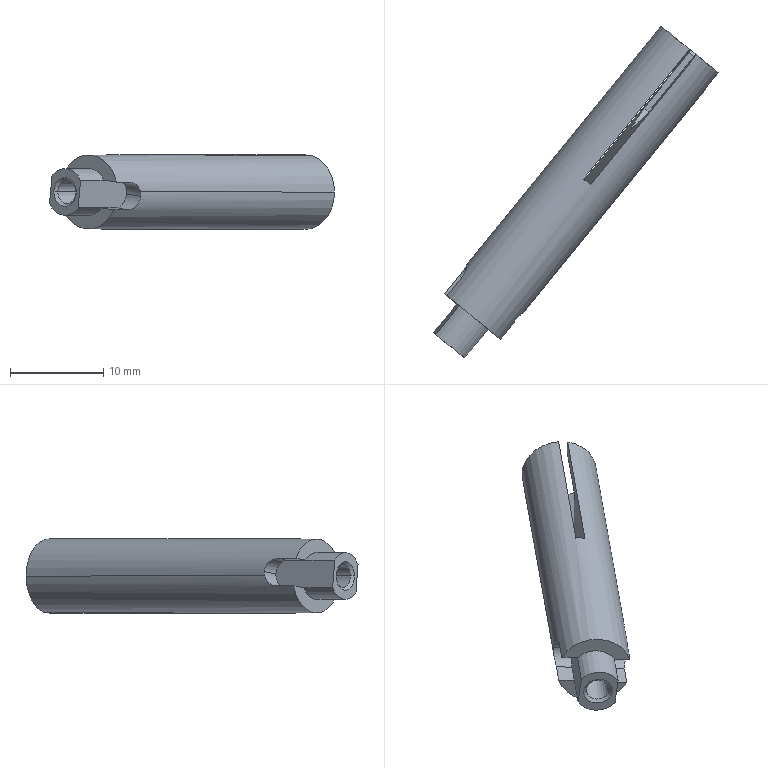Part | SolidWorks | features BaseBody 1 | 1 solid | 39 faces | box 30.645 x 35.694 x 8 mm | volume 1475 mm3 | plane 14 | cylinder 13 | cone 10 | spline 2 | commonest cylinder face diameters 3 x4 6 x3 2.5 x2 5 x2 8 x2
STEP:
#1=CARTESIAN_POINT('',(540.128,-144.913,299.195));
#2=VERTEX_POINT('',#1);
#3=CARTESIAN_POINT('',(538.707,-143.757,300.301));
#4=VERTEX_POINT('',#3);
#5=CARTESIAN_POINT('',(539.158,-144.124,299.195));
#6=DIRECTION('',(-0.6309,-0.7758,0.000000012));
#7=DIRECTION('',(0.7758,-0.6309,0.));
#8=AXIS2_PLACEMENT_3D('',#5,#6,#7);
#9=CIRCLE('',#8,1.25);
#10=EDGE_CURVE('',#2,#4,#9,.T.);
#11=ORIENTED_EDGE('',*,*,#10,.T.);
#12=CARTESIAN_POINT('',(539.969,-142.205,300.301));
#13=VERTEX_POINT('',#12);
#14=CARTESIAN_POINT('',(538.707,-143.757,300.301));
#15=CARTESIAN_POINT('',(539.969,-142.205,300.301));
#16=B_SPLINE_CURVE_WITH_KNOTS('',1,(#14,#15),.UNSPECIFIED.,.F.,.F.,(2,2),(0.,1.),.UNSPECIFIED.);
#17=EDGE_CURVE('',#4,#13,#16,.T.);
#18=ORIENTED_EDGE('',*,*,#17,.T.);
#19=CARTESIAN_POINT('',(541.39,-143.361,299.195));
#20=VERTEX_POINT('',#19);
#21=CARTESIAN_POINT('',(540.42,-142.572,299.195));
#22=DIRECTION('',(-0.6309,-0.7758,0.000000012));
#23=DIRECTION('',(0.7758,-0.6309,0.));
#24=AXIS2_PLACEMENT_3D('',#21,#22,#23);
#25=CIRCLE('',#24,1.25);
#26=EDGE_CURVE('',#20,#13,#25,.T.);
#27=ORIENTED_EDGE('',*,*,#26,.F.);
#28=CARTESIAN_POINT('',(540.871,-142.939,298.088));
#29=VERTEX_POINT('',#28);
#30=CARTESIAN_POINT('',(540.42,-142.572,299.195));
#31=DIRECTION('',(-0.6309,-0.7758,0.000000012));
#32=DIRECTION('',(0.7758,-0.6309,0.));
#33=AXIS2_PLACEMENT_3D('',#30,#31,#32);
#34=CIRCLE('',#33,1.25);
#35=EDGE_CURVE('',#29,#20,#34,.T.);
#36=ORIENTED_EDGE('',*,*,#35,.F.);
#37=CARTESIAN_POINT('',(539.609,-144.491,298.088));
#38=VERTEX_POINT('',#37);
#39=CARTESIAN_POINT('',(539.609,-144.491,298.088));
#40=CARTESIAN_POINT('',(540.871,-142.939,298.088));
#41=B_SPLINE_CURVE_WITH_KNOTS('',1,(#39,#40),.UNSPECIFIED.,.F.,.F.,(2,2),(0.,1.),.UNSPECIFIED.);
#42=EDGE_CURVE('',#38,#29,#41,.T.);
#43=ORIENTED_EDGE('',*,*,#42,.F.);
#44=CARTESIAN_POINT('',(539.158,-144.124,299.195));
#45=DIRECTION('',(-0.6309,-0.7758,0.000000012));
#46=DIRECTION('',(0.7758,-0.6309,0.));
#47=AXIS2_PLACEMENT_3D('',#44,#45,#46);
#48=CIRCLE('',#47,1.25);
#49=EDGE_CURVE('',#38,#2,#48,.T.);
#50=ORIENTED_EDGE('',*,*,#49,.T.);
#51=EDGE_LOOP('',(#11,#18,#27,#36,#43,#50));
#52=FACE_OUTER_BOUND('',#51,.T.);
#53=CARTESIAN_POINT('',(539.609,-144.491,298.088));
#54=CARTESIAN_POINT('',(541.326,-145.887,299.252));
#55=CARTESIAN_POINT('',(540.423,-145.153,301.464));
#56=CARTESIAN_POINT('',(538.707,-143.757,300.301));
#57=CARTESIAN_POINT('',(536.99,-142.361,299.138));
#58=CARTESIAN_POINT('',(537.892,-143.095,296.925));
#59=CARTESIAN_POINT('',(539.609,-144.491,298.088));
#60=CARTESIAN_POINT('',(540.871,-142.939,298.088));
#61=CARTESIAN_POINT('',(542.588,-144.335,299.252));
#62=CARTESIAN_POINT('',(541.685,-143.601,301.464));
#63=CARTESIAN_POINT('',(539.969,-142.205,300.301));
#64=CARTESIAN_POINT('',(538.252,-140.809,299.138));
#65=CARTESIAN_POINT('',(539.154,-141.543,296.925));
#66=CARTESIAN_POINT('',(540.871,-142.939,298.088));
#67=(BOUNDED_SURFACE()B_SPLINE_SURFACE(1,3,((#53,#54,#55,#56,#57,#58,#59),(#60,#61,#62,#63,#64,#65,#66)),.UNSPECIFIED.,.F.,.T.,.F.)B_SPLINE_SURFACE_WITH_KNOTS((2,2),(4,3,4),(0.,1.),(0.,0.5,1.),.UNSPECIFIED.)GEOMETRIC_REPRESENTATION_ITEM()RATIONAL_B_SPLINE_SURFACE(((1.,0.3333,0.3333,1.,0.3333,0.3333,1.),(1.,0.3333,0.3333,1.,0.3333,0.3333,1.)))REPRESENTATION_ITEM('')SURFACE());
#68=ADVANCED_FACE('',(#52),#67,.F.);
#69=CARTESIAN_POINT('',(538.678,-150.822,300.267));
#70=VERTEX_POINT('',#69);
#71=CARTESIAN_POINT('',(539.694,-149.805,299.195));
#72=VERTEX_POINT('',#71);
#73=CARTESIAN_POINT('',(538.678,-150.822,300.267));
#74=CARTESIAN_POINT('',(538.779,-150.697,300.267));
#75=CARTESIAN_POINT('',(538.884,-150.58,300.241));
#76=CARTESIAN_POINT('',(539.097,-150.361,300.137));
#77=CARTESIAN_POINT('',(539.2,-150.264,300.061));
#78=CARTESIAN_POINT('',(539.39,-150.09,299.868));
#79=CARTESIAN_POINT('',(539.474,-150.017,299.753));
#80=CARTESIAN_POINT('',(539.612,-149.891,299.491));
#81=CARTESIAN_POINT('',(539.664,-149.842,299.347));
#82=CARTESIAN_POINT('',(539.694,-149.805,299.195));
#83=B_SPLINE_CURVE_WITH_KNOTS('',3,(#73,#74,#75,#76,#77,#78,#79,#80,#81,#82),.UNSPECIFIED.,.F.,.F.,(4,2,2,2,4),(0.,0.0004777,0.0009554,0.001433,0.001911),.UNSPECIFIED.);
#84=EDGE_CURVE('',#70,#72,#83,.T.);
#85=ORIENTED_EDGE('',*,*,#84,.T.);
#86=CARTESIAN_POINT('',(560.558,-124.148,299.195));
#87=VERTEX_POINT('',#86);
#88=CARTESIAN_POINT('',(537.214,-152.854,299.195));
#89=DIRECTION('',(0.6309,0.7758,-0.000000012));
#90=VECTOR('',#89,1000.);
#91=LINE('',#88,#90);
#92=EDGE_CURVE('',#72,#87,#91,.T.);
#93=ORIENTED_EDGE('',*,*,#92,.T.);
#94=CARTESIAN_POINT('',(558.187,-122.22,303.082));
#95=VERTEX_POINT('',#94);
#96=CARTESIAN_POINT('',(557.455,-121.625,299.195));
#97=DIRECTION('',(-0.6309,-0.7758,0.000000012));
#98=DIRECTION('',(-0.7758,0.6309,0.));
#99=AXIS2_PLACEMENT_3D('',#96,#97,#98);
#100=CIRCLE('',#99,4.);
#101=EDGE_CURVE('',#87,#95,#100,.T.);
#102=ORIENTED_EDGE('',*,*,#101,.T.);
#103=CARTESIAN_POINT('',(546.831,-136.185,303.082));
#104=VERTEX_POINT('',#103);
#105=CARTESIAN_POINT('',(534.843,-150.926,303.082));
#106=DIRECTION('',(-0.6309,-0.7758,0.000000012));
#107=VECTOR('',#106,1000.);
#108=LINE('',#105,#107);
#109=EDGE_CURVE('',#95,#104,#108,.T.);
#110=ORIENTED_EDGE('',*,*,#109,.T.);
#111=CARTESIAN_POINT('',(546.06,-135.558,303.194));
#112=VERTEX_POINT('',#111);
#113=CARTESIAN_POINT('',(546.098,-135.59,299.195));
#114=DIRECTION('',(-0.6309,-0.7758,0.000000012));
#115=DIRECTION('',(-0.7758,0.6309,0.));
#116=AXIS2_PLACEMENT_3D('',#113,#114,#115);
#117=CIRCLE('',#116,4.);
#118=EDGE_CURVE('',#104,#112,#117,.T.);
#119=ORIENTED_EDGE('',*,*,#118,.T.);
#120=CARTESIAN_POINT('',(557.416,-121.593,303.194));
#121=VERTEX_POINT('',#120);
#122=CARTESIAN_POINT('',(534.072,-150.299,303.194));
#123=DIRECTION('',(0.6309,0.7758,-0.000000012));
#124=VECTOR('',#123,1000.);
#125=LINE('',#122,#124);
#126=EDGE_CURVE('',#112,#121,#125,.T.);
#127=ORIENTED_EDGE('',*,*,#126,.T.);
#128=CARTESIAN_POINT('',(554.352,-119.101,299.195));
#129=VERTEX_POINT('',#128);
#130=CARTESIAN_POINT('',(557.455,-121.625,299.195));
#131=DIRECTION('',(-0.6309,-0.7758,0.000000012));
#132=DIRECTION('',(-0.7758,0.6309,0.));
#133=AXIS2_PLACEMENT_3D('',#130,#131,#132);
#134=CIRCLE('',#133,4.);
#135=EDGE_CURVE('',#121,#129,#134,.T.);
#136=ORIENTED_EDGE('',*,*,#135,.T.);
#137=CARTESIAN_POINT('',(533.487,-144.757,299.195));
#138=VERTEX_POINT('',#137);
#139=CARTESIAN_POINT('',(531.007,-147.807,299.195));
#140=DIRECTION('',(0.6309,0.7758,-0.000000012));
#141=VECTOR('',#140,1000.);
#142=LINE('',#139,#141);
#143=EDGE_CURVE('',#138,#129,#142,.T.);
#144=ORIENTED_EDGE('',*,*,#143,.F.);
#145=CARTESIAN_POINT('',(533.551,-144.72,299.645));
#146=VERTEX_POINT('',#145);
#147=CARTESIAN_POINT('',(533.487,-144.757,299.195));
#148=CARTESIAN_POINT('',(533.516,-144.722,299.339));
#149=CARTESIAN_POINT('',(533.537,-144.709,299.492));
#150=CARTESIAN_POINT('',(533.551,-144.72,299.645));
#151=B_SPLINE_CURVE_WITH_KNOTS('',3,(#147,#148,#149,#150),.UNSPECIFIED.,.F.,.F.,(4,4),(0.0007269,0.001182),.UNSPECIFIED.);
#152=EDGE_CURVE('',#138,#146,#151,.T.);
#153=ORIENTED_EDGE('',*,*,#152,.T.);
#154=CARTESIAN_POINT('',(532.96,-146.173,301.103));
#155=VERTEX_POINT('',#154);
#156=CARTESIAN_POINT('',(533.551,-144.72,299.645));
#157=CARTESIAN_POINT('',(533.559,-144.727,299.745));
#158=CARTESIAN_POINT('',(533.565,-144.744,299.842));
#159=CARTESIAN_POINT('',(533.568,-144.796,300.032));
#160=CARTESIAN_POINT('',(533.566,-144.833,300.126));
#161=CARTESIAN_POINT('',(533.549,-144.965,300.391));
#162=CARTESIAN_POINT('',(533.522,-145.086,300.551));
#163=CARTESIAN_POINT('',(533.431,-145.365,300.815));
#164=CARTESIAN_POINT('',(533.366,-145.526,300.921));
#165=CARTESIAN_POINT('',(533.195,-145.85,301.064));
#166=CARTESIAN_POINT('',(533.087,-146.018,301.103));
#167=CARTESIAN_POINT('',(532.96,-146.173,301.103));
#168=B_SPLINE_CURVE_WITH_KNOTS('',3,(#156,#157,#158,#159,#160,#161,#162,#163,#164,#165,#166,#167),.UNSPECIFIED.,.F.,.F.,(4,2,2,2,2,4),(0.001182,0.001478,0.001774,0.002365,0.002957,0.003548),.UNSPECIFIED.);
#169=EDGE_CURVE('',#146,#155,#168,.T.);
#170=ORIENTED_EDGE('',*,*,#169,.T.);
#171=CARTESIAN_POINT('',(531.383,-148.113,301.103));
#172=VERTEX_POINT('',#171);
#173=CARTESIAN_POINT('',(531.383,-148.113,301.103));
#174=DIRECTION('',(-0.6309,-0.7758,0.000000012));
#175=VECTOR('',#174,1000.);
#176=LINE('',#173,#175);
#177=EDGE_CURVE('',#155,#172,#176,.T.);
#178=ORIENTED_EDGE('',*,*,#177,.T.);
#179=CARTESIAN_POINT('',(537.1,-152.762,300.267));
#180=VERTEX_POINT('',#179);
#181=CARTESIAN_POINT('',(534.111,-150.331,299.195));
#182=DIRECTION('',(0.6309,0.7758,-0.000000012));
#183=DIRECTION('',(-0.7758,0.6309,0.));
#184=AXIS2_PLACEMENT_3D('',#181,#182,#183);
#185=CIRCLE('',#184,4.);
#186=EDGE_CURVE('',#172,#180,#185,.T.);
#187=ORIENTED_EDGE('',*,*,#186,.T.);
#188=CARTESIAN_POINT('',(537.1,-152.762,300.267));
#189=DIRECTION('',(0.6309,0.7758,-0.000000012));
#190=VECTOR('',#189,1000.);
#191=LINE('',#188,#190);
#192=EDGE_CURVE('',#180,#70,#191,.T.);
#193=ORIENTED_EDGE('',*,*,#192,.T.);
#194=EDGE_LOOP('',(#85,#93,#102,#110,#119,#127,#136,#144,#153,#170,#178,#187,#193));
#195=FACE_OUTER_BOUND('',#194,.T.);
#196=CARTESIAN_POINT('',(534.111,-150.331,299.195));
#197=DIRECTION('',(0.6309,0.7758,-0.000000012));
#198=DIRECTION('',(-0.7758,0.6309,0.));
#199=AXIS2_PLACEMENT_3D('',#196,#197,#198);
#200=CYLINDRICAL_SURFACE('',#199,4.);
#201=ADVANCED_FACE('',(#195),#200,.T.);
#202=ORIENTED_EDGE('',*,*,#169,.F.);
#203=CARTESIAN_POINT('',(535.092,-145.974,299.42));
#204=VERTEX_POINT('',#203);
#205=CARTESIAN_POINT('',(534.08,-145.151,299.568));
#206=DIRECTION('',(0.7709,-0.6269,-0.1126));
#207=VECTOR('',#206,1000.);
#208=LINE('',#205,#207);
#209=EDGE_CURVE('',#146,#204,#208,.T.);
#210=ORIENTED_EDGE('',*,*,#209,.T.);
#211=CARTESIAN_POINT('',(534.277,-147.244,300.91));
#212=VERTEX_POINT('',#211);
#213=CARTESIAN_POINT('',(534.146,-147.137,299.42));
#214=DIRECTION('',(-0.7709,0.6269,0.1126));
#215=DIRECTION('',(0.6309,0.7758,0.));
#216=AXIS2_PLACEMENT_3D('',#213,#214,#215);
#217=CIRCLE('',#216,1.5);
#218=EDGE_CURVE('',#212,#204,#217,.T.);
#219=ORIENTED_EDGE('',*,*,#218,.F.);
#220=CARTESIAN_POINT('',(534.277,-147.244,300.91));
#221=DIRECTION('',(-0.7709,0.6269,0.1126));
#222=VECTOR('',#221,1000.);
#223=LINE('',#220,#222);
#224=EDGE_CURVE('',#212,#155,#223,.T.);
#225=ORIENTED_EDGE('',*,*,#224,.T.);
#226=EDGE_LOOP('',(#202,#210,#219,#225));
#227=FACE_OUTER_BOUND('',#226,.T.);
#228=CARTESIAN_POINT('',(533.134,-146.314,299.568));
#229=DIRECTION('',(0.7709,-0.6269,-0.1126));
#230=DIRECTION('',(0.6309,0.7758,0.));
#231=AXIS2_PLACEMENT_3D('',#228,#229,#230);
#232=CYLINDRICAL_SURFACE('',#231,1.5);
#233=ADVANCED_FACE('',(#227),#232,.F.);
#234=CARTESIAN_POINT('',(538.176,-148.481,298.969));
#235=VERTEX_POINT('',#234);
#236=CARTESIAN_POINT('',(537.361,-149.752,300.46));
#237=VERTEX_POINT('',#236);
#238=CARTESIAN_POINT('',(537.23,-149.645,298.969));
#239=DIRECTION('',(0.7709,-0.6269,-0.1126));
#240=DIRECTION('',(0.6309,0.7758,0.));
#241=AXIS2_PLACEMENT_3D('',#238,#239,#240);
#242=CIRCLE('',#241,1.5);
#243=EDGE_CURVE('',#235,#237,#242,.T.);
#244=ORIENTED_EDGE('',*,*,#243,.F.);
#245=CARTESIAN_POINT('',(539.718,-149.735,298.744));
#246=VERTEX_POINT('',#245);
#247=CARTESIAN_POINT('',(538.53,-148.769,298.918));
#248=DIRECTION('',(0.7709,-0.6269,-0.1126));
#249=VECTOR('',#248,1000.);
#250=LINE('',#247,#249);
#251=EDGE_CURVE('',#235,#246,#250,.T.);
#252=ORIENTED_EDGE('',*,*,#251,.T.);
#253=CARTESIAN_POINT('',(539.694,-149.805,299.195));
#254=CARTESIAN_POINT('',(539.723,-149.77,299.049));
#255=CARTESIAN_POINT('',(539.731,-149.746,298.897));
#256=CARTESIAN_POINT('',(539.718,-149.735,298.744));
#257=B_SPLINE_CURVE_WITH_KNOTS('',3,(#253,#254,#255,#256),.UNSPECIFIED.,.F.,.F.,(4,4),(0.001911,0.002365),.UNSPECIFIED.);
#258=EDGE_CURVE('',#72,#246,#257,.T.);
#259=ORIENTED_EDGE('',*,*,#258,.F.);
#260=ORIENTED_EDGE('',*,*,#84,.F.);
#261=CARTESIAN_POINT('',(537.714,-150.039,300.408));
#262=DIRECTION('',(0.7709,-0.6269,-0.1126));
#263=VECTOR('',#262,1000.);
#264=LINE('',#261,#263);
#265=EDGE_CURVE('',#237,#70,#264,.T.);
#266=ORIENTED_EDGE('',*,*,#265,.F.);
#267=EDGE_LOOP('',(#244,#252,#259,#260,#266));
#268=FACE_OUTER_BOUND('',#267,.T.);
#269=CARTESIAN_POINT('',(537.583,-149.933,298.918));
#270=DIRECTION('',(0.7709,-0.6269,-0.1126));
#271=DIRECTION('',(0.6309,0.7758,0.));
#272=AXIS2_PLACEMENT_3D('',#269,#270,#271);
#273=CYLINDRICAL_SURFACE('',#272,1.5);
#274=ADVANCED_FACE('',(#268),#273,.F.);
#275=CARTESIAN_POINT('',(557.91,-122.381,302.077));
#276=VERTEX_POINT('',#275);
#277=CARTESIAN_POINT('',(559.593,-123.75,299.195));
#278=VERTEX_POINT('',#277);
#279=CARTESIAN_POINT('',(557.266,-121.857,299.195));
#280=DIRECTION('',(0.6309,0.7758,-0.000000012));
#281=DIRECTION('',(0.361,-0.2936,-0.8851));
#282=AXIS2_PLACEMENT_3D('',#279,#280,#281);
#283=CIRCLE('',#282,3.);
#284=EDGE_CURVE('',#276,#278,#283,.T.);
#285=ORIENTED_EDGE('',*,*,#284,.T.);
#286=CARTESIAN_POINT('',(554.735,-129.724,299.195));
#287=VERTEX_POINT('',#286);
#288=CARTESIAN_POINT('',(557.259,-126.621,299.195));
#289=DIRECTION('',(-0.6309,-0.7758,0.000000012));
#290=VECTOR('',#289,1000.);
#291=LINE('',#288,#290);
#292=EDGE_CURVE('',#278,#287,#291,.T.);
#293=ORIENTED_EDGE('',*,*,#292,.T.);
#294=CARTESIAN_POINT('',(553.052,-128.355,302.077));
#295=VERTEX_POINT('',#294);
#296=CARTESIAN_POINT('',(552.408,-127.831,299.195));
#297=DIRECTION('',(0.6309,0.7758,-0.000000012));
#298=DIRECTION('',(0.7758,-0.6309,0.));
#299=AXIS2_PLACEMENT_3D('',#296,#297,#298);
#300=CIRCLE('',#299,3.);
#301=EDGE_CURVE('',#295,#287,#300,.T.);
#302=ORIENTED_EDGE('',*,*,#301,.F.);
#303=CARTESIAN_POINT('',(558.099,-122.148,302.077));
#304=DIRECTION('',(0.6309,0.7758,0.));
#305=VECTOR('',#304,1000.);
#306=LINE('',#303,#305);
#307=EDGE_CURVE('',#295,#276,#306,.T.);
#308=ORIENTED_EDGE('',*,*,#307,.T.);
#309=EDGE_LOOP('',(#285,#293,#302,#308));
#310=FACE_OUTER_BOUND('',#309,.T.);
#311=CARTESIAN_POINT('',(554.931,-124.728,299.195));
#312=DIRECTION('',(-0.6309,-0.7758,0.000000012));
#313=DIRECTION('',(0.7758,-0.6309,0.));
#314=AXIS2_PLACEMENT_3D('',#311,#312,#313);
#315=CYLINDRICAL_SURFACE('',#314,3.);
#316=ADVANCED_FACE('',(#310),#315,.F.);
#317=CARTESIAN_POINT('',(552.281,-127.728,302.19));
#318=VERTEX_POINT('',#317);
#319=CARTESIAN_POINT('',(550.442,-129.451,299.195));
#320=VERTEX_POINT('',#319);
#321=CARTESIAN_POINT('',(552.281,-127.728,302.19));
#322=CARTESIAN_POINT('',(551.946,-128.055,301.722));
#323=CARTESIAN_POINT('',(551.612,-128.381,301.254));
#324=CARTESIAN_POINT('',(551.118,-128.861,300.539));
#325=CARTESIAN_POINT('',(550.954,-129.02,300.3));
#326=CARTESIAN_POINT('',(550.718,-129.242,299.924));
#327=CARTESIAN_POINT('',(550.641,-129.314,299.796));
#328=CARTESIAN_POINT('',(550.538,-129.403,299.587));
#329=CARTESIAN_POINT('',(550.507,-129.428,299.515));
#330=CARTESIAN_POINT('',(550.459,-129.46,299.36));
#331=CARTESIAN_POINT('',(550.443,-129.464,299.276));
#332=CARTESIAN_POINT('',(550.442,-129.451,299.195));
#333=B_SPLINE_CURVE_WITH_KNOTS('',3,(#321,#322,#323,#324,#325,#326,#327,#328,#329,#330,#331,#332),.UNSPECIFIED.,.F.,.F.,(4,2,2,2,2,4),(-0.003068,-0.001082,-0.00008881,0.0004077,0.000656,0.0009043),.UNSPECIFIED.);
#334=EDGE_CURVE('',#318,#320,#333,.T.);
#335=ORIENTED_EDGE('',*,*,#334,.T.);
#336=CARTESIAN_POINT('',(550.08,-125.938,299.195));
#337=VERTEX_POINT('',#336);
#338=CARTESIAN_POINT('',(550.08,-125.938,299.195));
#339=DIRECTION('',(-0.1025,0.9947,-0.000000009));
#340=VECTOR('',#339,1000.);
#341=LINE('',#338,#340);
#342=EDGE_CURVE('',#320,#337,#341,.T.);
#343=ORIENTED_EDGE('',*,*,#342,.T.);
#344=CARTESIAN_POINT('',(552.408,-127.831,299.195));
#345=DIRECTION('',(0.6309,0.7758,-0.000000012));
#346=DIRECTION('',(0.7758,-0.6309,0.));
#347=AXIS2_PLACEMENT_3D('',#344,#345,#346);
#348=CIRCLE('',#347,3.);
#349=EDGE_CURVE('',#337,#318,#348,.T.);
#350=ORIENTED_EDGE('',*,*,#349,.T.);
#351=EDGE_LOOP('',(#335,#343,#350));
#352=FACE_OUTER_BOUND('',#351,.T.);
#353=CARTESIAN_POINT('',(552.408,-127.831,299.195));
#354=DIRECTION('',(0.6309,0.7758,-0.000000012));
#355=DIRECTION('',(-0.7758,0.6309,0.));
#356=AXIS2_PLACEMENT_3D('',#353,#354,#355);
#357=CONICAL_SURFACE('',#356,3.,0.7854);
#358=ADVANCED_FACE('',(#352),#357,.F.);
#359=CARTESIAN_POINT('',(557.139,-121.754,302.19));
#360=VERTEX_POINT('',#359);
#361=CARTESIAN_POINT('',(554.938,-119.964,299.195));
#362=VERTEX_POINT('',#361);
#363=CARTESIAN_POINT('',(557.266,-121.857,299.195));
#364=DIRECTION('',(-0.6309,-0.7758,0.000000012));
#365=DIRECTION('',(0.7758,-0.6309,0.));
#366=AXIS2_PLACEMENT_3D('',#363,#364,#365);
#367=CIRCLE('',#366,3.);
#368=EDGE_CURVE('',#360,#362,#367,.T.);
#369=ORIENTED_EDGE('',*,*,#368,.T.);
#370=CARTESIAN_POINT('',(554.895,-119.542,299.195));
#371=VERTEX_POINT('',#370);
#372=CARTESIAN_POINT('',(554.895,-119.542,299.195));
#373=DIRECTION('',(-0.1025,0.9947,-0.000000009));
#374=VECTOR('',#373,1000.);
#375=LINE('',#372,#374);
#376=EDGE_CURVE('',#362,#371,#375,.T.);
#377=ORIENTED_EDGE('',*,*,#376,.T.);
#378=CARTESIAN_POINT('',(557.355,-121.543,302.492));
#379=VERTEX_POINT('',#378);
#380=CARTESIAN_POINT('',(557.455,-121.625,299.195));
#381=DIRECTION('',(-0.6309,-0.7758,0.000000012));
#382=DIRECTION('',(-0.7758,0.6309,0.));
#383=AXIS2_PLACEMENT_3D('',#380,#381,#382);
#384=CIRCLE('',#383,3.3);
#385=EDGE_CURVE('',#379,#371,#384,.T.);
#386=ORIENTED_EDGE('',*,*,#385,.F.);
#387=CARTESIAN_POINT('',(557.139,-121.754,302.19));
#388=CARTESIAN_POINT('',(557.211,-121.684,302.291));
#389=CARTESIAN_POINT('',(557.283,-121.613,302.391));
#390=CARTESIAN_POINT('',(557.355,-121.543,302.492));
#391=B_SPLINE_CURVE_WITH_KNOTS('',3,(#387,#388,#389,#390),.UNSPECIFIED.,.F.,.F.,(4,4),(0.,0.000427),.UNSPECIFIED.);
#392=EDGE_CURVE('',#360,#379,#391,.T.);
#393=ORIENTED_EDGE('',*,*,#392,.F.);
#394=EDGE_LOOP('',(#369,#377,#386,#393));
#395=FACE_OUTER_BOUND('',#394,.T.);
#396=CARTESIAN_POINT('',(557.455,-121.625,299.195));
#397=DIRECTION('',(0.6309,0.7758,-0.000000012));
#398=DIRECTION('',(-0.7758,0.6309,0.));
#399=AXIS2_PLACEMENT_3D('',#396,#397,#398);
#400=CONICAL_SURFACE('',#399,3.3,0.7854);
#401=ADVANCED_FACE('',(#395),#400,.F.);
#402=CARTESIAN_POINT('',(530.806,-152.413,299.195));
#403=VERTEX_POINT('',#402);
#404=CARTESIAN_POINT('',(532.746,-153.99,299.195));
#405=VERTEX_POINT('',#404);
#406=CARTESIAN_POINT('',(531.776,-153.201,299.195));
#407=DIRECTION('',(-0.6309,-0.7758,0.000000012));
#408=DIRECTION('',(-0.361,0.2936,0.8851));
#409=AXIS2_PLACEMENT_3D('',#406,#407,#408);
#410=CIRCLE('',#409,1.25);
#411=EDGE_CURVE('',#403,#405,#410,.T.);
#412=ORIENTED_EDGE('',*,*,#411,.F.);
#413=CARTESIAN_POINT('',(530.384,-152.456,299.195));
#414=VERTEX_POINT('',#413);
#415=CARTESIAN_POINT('',(530.384,-152.456,299.195));
#416=DIRECTION('',(-0.9947,-0.1025,0.000000009));
#417=VECTOR('',#416,1000.);
#418=LINE('',#415,#417);
#419=EDGE_CURVE('',#403,#414,#418,.T.);
#420=ORIENTED_EDGE('',*,*,#419,.T.);
#421=CARTESIAN_POINT('',(532.789,-154.412,299.195));
#422=VERTEX_POINT('',#421);
#423=CARTESIAN_POINT('',(531.587,-153.434,299.195));
#424=DIRECTION('',(0.6309,0.7758,-0.000000012));
#425=DIRECTION('',(0.7758,-0.6309,0.));
#426=AXIS2_PLACEMENT_3D('',#423,#424,#425);
#427=CIRCLE('',#426,1.55);
#428=EDGE_CURVE('',#422,#414,#427,.T.);
#429=ORIENTED_EDGE('',*,*,#428,.F.);
#430=CARTESIAN_POINT('',(532.789,-154.412,299.195));
#431=DIRECTION('',(0.1025,-0.9947,0.000000009));
#432=VECTOR('',#431,1000.);
#433=LINE('',#430,#432);
#434=EDGE_CURVE('',#405,#422,#433,.T.);
#435=ORIENTED_EDGE('',*,*,#434,.F.);
#436=EDGE_LOOP('',(#412,#420,#429,#435));
#437=FACE_OUTER_BOUND('',#436,.T.);
#438=CARTESIAN_POINT('',(531.587,-153.434,299.195));
#439=DIRECTION('',(-0.6309,-0.7758,0.000000012));
#440=DIRECTION('',(0.7758,-0.6309,0.));
#441=AXIS2_PLACEMENT_3D('',#438,#439,#440);
#442=CONICAL_SURFACE('',#441,1.55,0.7854);
#443=ADVANCED_FACE('',(#437),#442,.F.);
#444=CARTESIAN_POINT('',(538.188,-143.335,299.195));
#445=VERTEX_POINT('',#444);
#446=CARTESIAN_POINT('',(539.158,-144.124,299.195));
#447=DIRECTION('',(-0.6309,-0.7758,0.000000012));
#448=DIRECTION('',(0.7758,-0.6309,0.));
#449=AXIS2_PLACEMENT_3D('',#446,#447,#448);
#450=CIRCLE('',#449,1.25);
#451=EDGE_CURVE('',#445,#38,#450,.T.);
#452=ORIENTED_EDGE('',*,*,#451,.F.);
#453=CARTESIAN_POINT('',(534.403,-147.99,299.195));
#454=DIRECTION('',(-0.6309,-0.7758,0.000000012));
#455=VECTOR('',#454,1000.);
#456=LINE('',#453,#455);
#457=EDGE_CURVE('',#445,#403,#456,.T.);
#458=ORIENTED_EDGE('',*,*,#457,.T.);
#459=ORIENTED_EDGE('',*,*,#411,.T.);
#460=CARTESIAN_POINT('',(536.342,-149.568,299.195));
#461=DIRECTION('',(-0.6309,-0.7758,0.000000012));
#462=VECTOR('',#461,1000.);
#463=LINE('',#460,#462);
#464=EDGE_CURVE('',#2,#405,#463,.T.);
#465=ORIENTED_EDGE('',*,*,#464,.F.);
#466=ORIENTED_EDGE('',*,*,#49,.F.);
#467=EDGE_LOOP('',(#452,#458,#459,#465,#466));
#468=FACE_OUTER_BOUND('',#467,.T.);
#469=CARTESIAN_POINT('',(535.372,-148.779,299.195));
#470=DIRECTION('',(-0.6309,-0.7758,0.000000012));
#471=DIRECTION('',(0.7758,-0.6309,0.));
#472=AXIS2_PLACEMENT_3D('',#469,#470,#471);
#473=CYLINDRICAL_SURFACE('',#472,1.25);
#474=ADVANCED_FACE('',(#468),#473,.F.);
#475=CARTESIAN_POINT('',(540.894,-141.99,299.195));
#476=VERTEX_POINT('',#475);
#477=CARTESIAN_POINT('',(541.39,-143.361,299.195));
#478=DIRECTION('',(0.3401,-0.9404,0.000000006));
#479=VECTOR('',#478,1000.);
#480=LINE('',#477,#479);
#481=EDGE_CURVE('',#476,#20,#480,.T.);
#482=ORIENTED_EDGE('',*,*,#481,.F.);
#483=CARTESIAN_POINT('',(539.45,-141.784,299.195));
#484=VERTEX_POINT('',#483);
#485=CARTESIAN_POINT('',(539.45,-141.784,299.195));
#486=DIRECTION('',(-0.99,0.1412,0.000000006));
#487=VECTOR('',#486,1000.);
#488=LINE('',#485,#487);
#489=EDGE_CURVE('',#476,#484,#488,.T.);
#490=ORIENTED_EDGE('',*,*,#489,.T.);
#491=CARTESIAN_POINT('',(540.42,-142.572,299.195));
#492=DIRECTION('',(-0.6309,-0.7758,0.000000012));
#493=DIRECTION('',(0.7758,-0.6309,0.));
#494=AXIS2_PLACEMENT_3D('',#491,#492,#493);
#495=CIRCLE('',#494,1.25);
#496=EDGE_CURVE('',#484,#29,#495,.T.);
#497=ORIENTED_EDGE('',*,*,#496,.T.);
#498=ORIENTED_EDGE('',*,*,#35,.T.);
#499=EDGE_LOOP('',(#482,#490,#497,#498));
#500=FACE_OUTER_BOUND('',#499,.T.);
#501=CARTESIAN_POINT('',(540.42,-142.572,299.195));
#502=DIRECTION('',(-0.6309,-0.7758,0.000000012));
#503=DIRECTION('',(0.7758,-0.6309,0.));
#504=AXIS2_PLACEMENT_3D('',#501,#502,#503);
#505=CONICAL_SURFACE('',#504,1.25,1.03);
#506=ADVANCED_FACE('',(#500),#505,.F.);
#507=ORIENTED_EDGE('',*,*,#92,.F.);
#508=ORIENTED_EDGE('',*,*,#258,.T.);
#509=CARTESIAN_POINT('',(538.415,-150.609,297.286));
#510=VERTEX_POINT('',#509);
#511=CARTESIAN_POINT('',(539.718,-149.735,298.744));
#512=CARTESIAN_POINT('',(539.709,-149.728,298.645));
#513=CARTESIAN_POINT('',(539.691,-149.726,298.548));
#514=CARTESIAN_POINT('',(539.639,-149.734,298.358));
#515=CARTESIAN_POINT('',(539.604,-149.743,298.264));
#516=CARTESIAN_POINT('',(539.478,-149.787,297.998));
#517=CARTESIAN_POINT('',(539.366,-149.837,297.839));
#518=CARTESIAN_POINT('',(539.173,-149.948,297.639));
#519=CARTESIAN_POINT('',(539.105,-149.99,297.58));
#520=CARTESIAN_POINT('',(538.967,-150.085,297.477));
#521=CARTESIAN_POINT('',(538.895,-150.139,297.432));
#522=CARTESIAN_POINT('',(538.682,-150.315,297.324));
#523=CARTESIAN_POINT('',(538.541,-150.454,297.286));
#524=CARTESIAN_POINT('',(538.415,-150.609,297.286));
#525=B_SPLINE_CURVE_WITH_KNOTS('',3,(#511,#512,#513,#514,#515,#516,#517,#518,#519,#520,#521,#522,#523,#524),.UNSPECIFIED.,.F.,.F.,(4,2,2,2,2,2,4),(0.002365,0.002661,0.002956,0.003547,0.003842,0.004138,0.004729),.UNSPECIFIED.);
#526=EDGE_CURVE('',#246,#510,#525,.T.);
#527=ORIENTED_EDGE('',*,*,#526,.T.);
#528=CARTESIAN_POINT('',(536.838,-152.549,297.286));
#529=VERTEX_POINT('',#528);
#530=CARTESIAN_POINT('',(536.838,-152.549,297.286));
#531=DIRECTION('',(-0.6309,-0.7758,0.000000012));
#532=VECTOR('',#531,1000.);
#533=LINE('',#530,#532);
#534=EDGE_CURVE('',#510,#529,#533,.T.);
#535=ORIENTED_EDGE('',*,*,#534,.T.);
#536=CARTESIAN_POINT('',(531.121,-147.899,298.122));
#537=VERTEX_POINT('',#536);
#538=CARTESIAN_POINT('',(534.111,-150.331,299.195));
#539=DIRECTION('',(0.6309,0.7758,-0.000000012));
#540=DIRECTION('',(-0.7758,0.6309,0.));
#541=AXIS2_PLACEMENT_3D('',#538,#539,#540);
#542=CIRCLE('',#541,4.);
#543=EDGE_CURVE('',#529,#537,#542,.T.);
#544=ORIENTED_EDGE('',*,*,#543,.T.);
#545=CARTESIAN_POINT('',(532.698,-145.96,298.122));
#546=VERTEX_POINT('',#545);
#547=CARTESIAN_POINT('',(531.121,-147.899,298.122));
#548=DIRECTION('',(0.6309,0.7758,-0.000000012));
#549=VECTOR('',#548,1000.);
#550=LINE('',#547,#549);
#551=EDGE_CURVE('',#537,#546,#550,.T.);
#552=ORIENTED_EDGE('',*,*,#551,.T.);
#553=CARTESIAN_POINT('',(532.698,-145.96,298.122));
#554=CARTESIAN_POINT('',(532.8,-145.835,298.122));
#555=CARTESIAN_POINT('',(532.893,-145.708,298.148));
#556=CARTESIAN_POINT('',(533.064,-145.456,298.252));
#557=CARTESIAN_POINT('',(533.138,-145.336,298.327));
#558=CARTESIAN_POINT('',(533.269,-145.114,298.52));
#559=CARTESIAN_POINT('',(533.325,-145.015,298.637));
#560=CARTESIAN_POINT('',(533.419,-144.856,298.897));
#561=CARTESIAN_POINT('',(533.457,-144.794,299.043));
#562=CARTESIAN_POINT('',(533.487,-144.757,299.195));
#563=B_SPLINE_CURVE_WITH_KNOTS('',3,(#553,#554,#555,#556,#557,#558,#559,#560,#561,#562),.UNSPECIFIED.,.F.,.F.,(4,2,2,2,4),(-0.001182,-0.0007049,-0.0002277,0.0002496,0.0007269),.UNSPECIFIED.);
#564=EDGE_CURVE('',#546,#138,#563,.T.);
#565=ORIENTED_EDGE('',*,*,#564,.T.);
#566=ORIENTED_EDGE('',*,*,#143,.T.);
#567=CARTESIAN_POINT('',(556.723,-121.029,295.308));
#568=VERTEX_POINT('',#567);
#569=CARTESIAN_POINT('',(557.455,-121.625,299.195));
#570=DIRECTION('',(-0.6309,-0.7758,0.000000012));
#571=DIRECTION('',(-0.7758,0.6309,0.));
#572=AXIS2_PLACEMENT_3D('',#569,#570,#571);
#573=CIRCLE('',#572,4.);
#574=EDGE_CURVE('',#129,#568,#573,.T.);
#575=ORIENTED_EDGE('',*,*,#574,.T.);
#576=CARTESIAN_POINT('',(545.366,-134.994,295.308));
#577=VERTEX_POINT('',#576);
#578=CARTESIAN_POINT('',(533.378,-149.735,295.308));
#579=DIRECTION('',(-0.6309,-0.7758,0.000000012));
#580=VECTOR('',#579,1000.);
#581=LINE('',#578,#580);
#582=EDGE_CURVE('',#568,#577,#581,.T.);
#583=ORIENTED_EDGE('',*,*,#582,.T.);
#584=CARTESIAN_POINT('',(546.137,-135.621,295.195));
#585=VERTEX_POINT('',#584);
#586=CARTESIAN_POINT('',(546.098,-135.59,299.195));
#587=DIRECTION('',(-0.6309,-0.7758,0.000000012));
#588=DIRECTION('',(-0.7758,0.6309,0.));
#589=AXIS2_PLACEMENT_3D('',#586,#587,#588);
#590=CIRCLE('',#589,4.);
#591=EDGE_CURVE('',#577,#585,#590,.T.);
#592=ORIENTED_EDGE('',*,*,#591,.T.);
#593=CARTESIAN_POINT('',(557.494,-121.656,295.195));
#594=VERTEX_POINT('',#593);
#595=CARTESIAN_POINT('',(534.149,-150.362,295.195));
#596=DIRECTION('',(0.6309,0.7758,-0.000000012));
#597=VECTOR('',#596,1000.);
#598=LINE('',#595,#597);
#599=EDGE_CURVE('',#585,#594,#598,.T.);
#600=ORIENTED_EDGE('',*,*,#599,.T.);
#601=CARTESIAN_POINT('',(557.455,-121.625,299.195));
#602=DIRECTION('',(-0.6309,-0.7758,0.000000012));
#603=DIRECTION('',(-0.7758,0.6309,0.));
#604=AXIS2_PLACEMENT_3D('',#601,#602,#603);
#605=CIRCLE('',#604,4.);
#606=EDGE_CURVE('',#594,#87,#605,.T.);
#607=ORIENTED_EDGE('',*,*,#606,.T.);
#608=EDGE_LOOP('',(#507,#508,#527,#535,#544,#552,#565,#566,#575,#583,#592,#600,#607));
#609=FACE_OUTER_BOUND('',#608,.T.);
#610=CARTESIAN_POINT('',(534.111,-150.331,299.195));
#611=DIRECTION('',(0.6309,0.7758,-0.000000012));
#612=DIRECTION('',(-0.7758,0.6309,0.));
#613=AXIS2_PLACEMENT_3D('',#610,#611,#612);
#614=CYLINDRICAL_SURFACE('',#613,4.);
#615=ADVANCED_FACE('',(#609),#614,.T.);
#616=CARTESIAN_POINT('',(535.784,-151.691,300.46));
#617=VERTEX_POINT('',#616);
#618=CARTESIAN_POINT('',(535.784,-151.691,300.46));
#619=DIRECTION('',(0.7709,-0.6269,-0.1126));
#620=VECTOR('',#619,1000.);
#621=LINE('',#618,#620);
#622=EDGE_CURVE('',#617,#180,#621,.T.);
#623=ORIENTED_EDGE('',*,*,#622,.T.);
#624=ORIENTED_EDGE('',*,*,#186,.F.);
#625=CARTESIAN_POINT('',(532.7,-149.183,300.91));
#626=VERTEX_POINT('',#625);
#627=CARTESIAN_POINT('',(532.7,-149.183,300.91));
#628=DIRECTION('',(-0.7709,0.6269,0.1126));
#629=VECTOR('',#628,1000.);
#630=LINE('',#627,#629);
#631=EDGE_CURVE('',#626,#172,#630,.T.);
#632=ORIENTED_EDGE('',*,*,#631,.F.);
#633=CARTESIAN_POINT('',(534.111,-150.331,299.195));
#634=DIRECTION('',(-0.6309,-0.7758,0.000000012));
#635=DIRECTION('',(0.7758,-0.6309,0.));
#636=AXIS2_PLACEMENT_3D('',#633,#634,#635);
#637=CIRCLE('',#636,2.5);
#638=EDGE_CURVE('',#617,#626,#637,.T.);
#639=ORIENTED_EDGE('',*,*,#638,.F.);
#640=EDGE_LOOP('',(#623,#624,#632,#639));
#641=FACE_OUTER_BOUND('',#640,.T.);
#642=CARTESIAN_POINT('',(534.111,-150.331,299.195));
#643=DIRECTION('',(0.6309,0.7758,-0.000000012));
#644=DIRECTION('',(-0.7758,0.6309,0.));
#645=AXIS2_PLACEMENT_3D('',#642,#643,#644);
#646=PLANE('',#645);
#647=ADVANCED_FACE('',(#641),#646,.F.);
#648=CARTESIAN_POINT('',(532.7,-149.183,300.91));
#649=DIRECTION('',(0.6309,0.7758,-0.000000012));
#650=VECTOR('',#649,1000.);
#651=LINE('',#648,#650);
#652=EDGE_CURVE('',#626,#212,#651,.T.);
#653=ORIENTED_EDGE('',*,*,#652,.F.);
#654=ORIENTED_EDGE('',*,*,#631,.T.);
#655=ORIENTED_EDGE('',*,*,#177,.F.);
#656=ORIENTED_EDGE('',*,*,#224,.F.);
#657=EDGE_LOOP('',(#653,#654,#655,#656));
#658=FACE_OUTER_BOUND('',#657,.T.);
#659=CARTESIAN_POINT('',(530.176,-152.287,300.91));
#660=DIRECTION('',(0.0874,-0.07107,0.9936));
#661=DIRECTION('',(0.9962,0.,-0.08762));
#662=AXIS2_PLACEMENT_3D('',#659,#660,#661);
#663=PLANE('',#662);
#664=ADVANCED_FACE('',(#658),#663,.F.);
#665=ORIENTED_EDGE('',*,*,#209,.F.);
#666=ORIENTED_EDGE('',*,*,#152,.F.);
#667=ORIENTED_EDGE('',*,*,#564,.F.);
#668=CARTESIAN_POINT('',(534.015,-147.031,297.929));
#669=VERTEX_POINT('',#668);
#670=CARTESIAN_POINT('',(532.698,-145.96,298.122));
#671=DIRECTION('',(0.7709,-0.6269,-0.1126));
#672=VECTOR('',#671,1000.);
#673=LINE('',#670,#672);
#674=EDGE_CURVE('',#546,#669,#673,.T.);
#675=ORIENTED_EDGE('',*,*,#674,.T.);
#676=CARTESIAN_POINT('',(534.146,-147.137,299.42));
#677=DIRECTION('',(-0.7709,0.6269,0.1126));
#678=DIRECTION('',(0.6309,0.7758,0.));
#679=AXIS2_PLACEMENT_3D('',#676,#677,#678);
#680=CIRCLE('',#679,1.5);
#681=EDGE_CURVE('',#204,#669,#680,.T.);
#682=ORIENTED_EDGE('',*,*,#681,.F.);
#683=EDGE_LOOP('',(#665,#666,#667,#675,#682));
#684=FACE_OUTER_BOUND('',#683,.T.);
#685=CARTESIAN_POINT('',(533.134,-146.314,299.568));
#686=DIRECTION('',(0.7709,-0.6269,-0.1126));
#687=DIRECTION('',(0.6309,0.7758,0.));
#688=AXIS2_PLACEMENT_3D('',#685,#686,#687);
#689=CYLINDRICAL_SURFACE('',#688,1.5);
#690=ADVANCED_FACE('',(#684),#689,.F.);
#691=ORIENTED_EDGE('',*,*,#551,.F.);
#692=CARTESIAN_POINT('',(532.438,-148.97,297.929));
#693=VERTEX_POINT('',#692);
#694=CARTESIAN_POINT('',(532.438,-148.97,297.929));
#695=DIRECTION('',(-0.7709,0.6269,0.1126));
#696=VECTOR('',#695,1000.);
#697=LINE('',#694,#696);
#698=EDGE_CURVE('',#693,#537,#697,.T.);
#699=ORIENTED_EDGE('',*,*,#698,.F.);
#700=CARTESIAN_POINT('',(534.015,-147.031,297.929));
#701=DIRECTION('',(-0.6309,-0.7758,0.000000012));
#702=VECTOR('',#701,1000.);
#703=LINE('',#700,#702);
#704=EDGE_CURVE('',#669,#693,#703,.T.);
#705=ORIENTED_EDGE('',*,*,#704,.F.);
#706=ORIENTED_EDGE('',*,*,#674,.F.);
#707=EDGE_LOOP('',(#691,#699,#705,#706));
#708=FACE_OUTER_BOUND('',#707,.T.);
#709=CARTESIAN_POINT('',(528.597,-151.003,298.122));
#710=DIRECTION('',(-0.0874,0.07107,-0.9936));
#711=DIRECTION('',(-0.9962,0.,0.08762));
#712=AXIS2_PLACEMENT_3D('',#709,#710,#711);
#713=PLANE('',#712);
#714=ADVANCED_FACE('',(#708),#713,.F.);
#715=CARTESIAN_POINT('',(535.521,-151.478,297.479));
#716=VERTEX_POINT('',#715);
#717=CARTESIAN_POINT('',(536.838,-152.549,297.286));
#718=DIRECTION('',(-0.7709,0.6269,0.1126));
#719=VECTOR('',#718,1000.);
#720=LINE('',#717,#719);
#721=EDGE_CURVE('',#529,#716,#720,.T.);
#722=ORIENTED_EDGE('',*,*,#721,.T.);
#723=CARTESIAN_POINT('',(534.111,-150.331,299.195));
#724=DIRECTION('',(-0.6309,-0.7758,0.000000012));
#725=DIRECTION('',(0.7758,-0.6309,0.));
#726=AXIS2_PLACEMENT_3D('',#723,#724,#725);
#727=CIRCLE('',#726,2.5);
#728=EDGE_CURVE('',#693,#716,#727,.T.);
#729=ORIENTED_EDGE('',*,*,#728,.F.);
#730=ORIENTED_EDGE('',*,*,#698,.T.);
#731=ORIENTED_EDGE('',*,*,#543,.F.);
#732=EDGE_LOOP('',(#722,#729,#730,#731));
#733=FACE_OUTER_BOUND('',#732,.T.);
#734=CARTESIAN_POINT('',(534.111,-150.331,299.195));
#735=DIRECTION('',(0.6309,0.7758,-0.000000012));
#736=DIRECTION('',(-0.7758,0.6309,0.));
#737=AXIS2_PLACEMENT_3D('',#734,#735,#736);
#738=PLANE('',#737);
#739=ADVANCED_FACE('',(#733),#738,.F.);
#740=CARTESIAN_POINT('',(557.555,-121.706,295.897));
#741=VERTEX_POINT('',#740);
#742=CARTESIAN_POINT('',(557.494,-121.656,295.195));
#743=DIRECTION('',(0.0874,-0.07107,0.9936));
#744=VECTOR('',#743,1000.);
#745=LINE('',#742,#744);
#746=EDGE_CURVE('',#594,#741,#745,.T.);
#747=ORIENTED_EDGE('',*,*,#746,.T.);
#748=CARTESIAN_POINT('',(558.126,-122.17,302.379));
#749=VERTEX_POINT('',#748);
#750=CARTESIAN_POINT('',(557.455,-121.625,299.195));
#751=DIRECTION('',(-0.6309,-0.7758,0.000000012));
#752=DIRECTION('',(-0.7758,0.6309,0.));
#753=AXIS2_PLACEMENT_3D('',#750,#751,#752);
#754=CIRCLE('',#753,3.3);
#755=EDGE_CURVE('',#741,#749,#754,.T.);
#756=ORIENTED_EDGE('',*,*,#755,.T.);
#757=CARTESIAN_POINT('',(558.126,-122.17,302.379));
#758=DIRECTION('',(0.0874,-0.07107,0.9936));
#759=VECTOR('',#758,1000.);
#760=LINE('',#757,#759);
#761=EDGE_CURVE('',#749,#95,#760,.T.);
#762=ORIENTED_EDGE('',*,*,#761,.T.);
#763=ORIENTED_EDGE('',*,*,#101,.F.);
#764=ORIENTED_EDGE('',*,*,#606,.F.);
#765=EDGE_LOOP('',(#747,#756,#762,#763,#764));
#766=FACE_OUTER_BOUND('',#765,.T.);
#767=CARTESIAN_POINT('',(557.455,-121.625,299.195));
#768=DIRECTION('',(0.6309,0.7758,-0.000000012));
#769=DIRECTION('',(-0.7758,0.6309,0.));
#770=AXIS2_PLACEMENT_3D('',#767,#768,#769);
#771=PLANE('',#770);
#772=ADVANCED_FACE('',(#766),#771,.T.);
#773=ORIENTED_EDGE('',*,*,#307,.F.);
#774=CARTESIAN_POINT('',(552.535,-127.934,296.199));
#775=VERTEX_POINT('',#774);
#776=CARTESIAN_POINT('',(552.535,-127.934,296.199));
#777=CARTESIAN_POINT('',(552.286,-128.324,296.662));
#778=CARTESIAN_POINT('',(552.037,-128.713,297.125));
#779=CARTESIAN_POINT('',(551.672,-129.288,297.831));
#780=CARTESIAN_POINT('',(551.551,-129.479,298.067));
#781=CARTESIAN_POINT('',(551.382,-129.753,298.438));
#782=CARTESIAN_POINT('',(551.328,-129.843,298.564));
#783=CARTESIAN_POINT('',(551.26,-129.963,298.767));
#784=CARTESIAN_POINT('',(551.24,-130.,298.838));
#785=CARTESIAN_POINT('',(551.214,-130.06,298.988));
#786=CARTESIAN_POINT('',(551.208,-130.081,299.068));
#787=CARTESIAN_POINT('',(551.225,-130.089,299.232));
#788=CARTESIAN_POINT('',(551.247,-130.077,299.312));
#789=CARTESIAN_POINT('',(551.302,-130.036,299.46));
#790=CARTESIAN_POINT('',(551.335,-130.008,299.529));
#791=CARTESIAN_POINT('',(551.438,-129.917,299.729));
#792=CARTESIAN_POINT('',(551.515,-129.845,299.854));
#793=CARTESIAN_POINT('',(551.748,-129.624,300.221));
#794=CARTESIAN_POINT('',(551.909,-129.468,300.456));
#795=CARTESIAN_POINT('',(552.395,-128.997,301.157));
#796=CARTESIAN_POINT('',(552.723,-128.676,301.618));
#797=CARTESIAN_POINT('',(553.052,-128.355,302.077));
#798=B_SPLINE_CURVE_WITH_KNOTS('',3,(#776,#777,#778,#779,#780,#781,#782,#783,#784,#785,#786,#787,#788,#789,#790,#791,#792,#793,#794,#795,#796,#797),.UNSPECIFIED.,.F.,.F.,(4,2,2,2,2,2,2,2,2,2,4),(-0.003068,-0.001104,-0.0001222,0.0003688,0.0006143,0.0008598,0.001105,0.001351,0.001842,0.002824,0.004788),.UNSPECIFIED.);
#799=EDGE_CURVE('',#775,#295,#798,.T.);
#800=ORIENTED_EDGE('',*,*,#799,.F.);
#801=CARTESIAN_POINT('',(557.393,-121.96,296.199));
#802=VERTEX_POINT('',#801);
#803=CARTESIAN_POINT('',(557.582,-121.728,296.199));
#804=DIRECTION('',(-0.6309,-0.7758,0.));
#805=VECTOR('',#804,1000.);
#806=LINE('',#803,#805);
#807=EDGE_CURVE('',#802,#775,#806,.T.);
#808=ORIENTED_EDGE('',*,*,#807,.F.);
#809=CARTESIAN_POINT('',(557.555,-121.706,295.897));
#810=CARTESIAN_POINT('',(557.501,-121.791,295.998));
#811=CARTESIAN_POINT('',(557.447,-121.876,296.098));
#812=CARTESIAN_POINT('',(557.393,-121.96,296.199));
#813=B_SPLINE_CURVE_WITH_KNOTS('',3,(#809,#810,#811,#812),.UNSPECIFIED.,.F.,.F.,(4,4),(0.,0.000427),.UNSPECIFIED.);
#814=EDGE_CURVE('',#741,#802,#813,.T.);
#815=ORIENTED_EDGE('',*,*,#814,.F.);
#816=ORIENTED_EDGE('',*,*,#746,.F.);
#817=ORIENTED_EDGE('',*,*,#599,.F.);
#818=CARTESIAN_POINT('',(546.831,-136.185,303.082));
#819=DIRECTION('',(-0.0874,0.07107,-0.9936));
#820=VECTOR('',#819,1000.);
#821=LINE('',#818,#820);
#822=EDGE_CURVE('',#104,#585,#821,.T.);
#823=ORIENTED_EDGE('',*,*,#822,.F.);
#824=ORIENTED_EDGE('',*,*,#109,.F.);
#825=ORIENTED_EDGE('',*,*,#761,.F.);
#826=CARTESIAN_POINT('',(557.91,-122.381,302.077));
#827=CARTESIAN_POINT('',(557.982,-122.311,302.178));
#828=CARTESIAN_POINT('',(558.054,-122.24,302.279));
#829=CARTESIAN_POINT('',(558.126,-122.17,302.379));
#830=B_SPLINE_CURVE_WITH_KNOTS('',3,(#826,#827,#828,#829),.UNSPECIFIED.,.F.,.F.,(4,4),(0.,0.000427),.UNSPECIFIED.);
#831=EDGE_CURVE('',#276,#749,#830,.T.);
#832=ORIENTED_EDGE('',*,*,#831,.F.);
#833=EDGE_LOOP('',(#773,#800,#808,#815,#816,#817,#823,#824,#825,#832));
#834=FACE_OUTER_BOUND('',#833,.T.);
#835=CARTESIAN_POINT('',(558.187,-122.22,303.082));
#836=DIRECTION('',(0.7709,-0.6269,-0.1126));
#837=DIRECTION('',(0.6309,0.7758,0.));
#838=AXIS2_PLACEMENT_3D('',#835,#836,#837);
#839=PLANE('',#838);
#840=ADVANCED_FACE('',(#834),#839,.F.);
#841=CARTESIAN_POINT('',(556.723,-121.029,295.308));
#842=DIRECTION('',(-0.0874,0.07107,-0.9936));
#843=VECTOR('',#842,1000.);
#844=LINE('',#841,#843);
#845=EDGE_CURVE('',#121,#379,#844,.T.);
#846=ORIENTED_EDGE('',*,*,#845,.F.);
#847=ORIENTED_EDGE('',*,*,#126,.F.);
#848=CARTESIAN_POINT('',(545.366,-134.994,295.308));
#849=DIRECTION('',(0.0874,-0.07107,0.9936));
#850=VECTOR('',#849,1000.);
#851=LINE('',#848,#850);
#852=EDGE_CURVE('',#577,#112,#851,.T.);
#853=ORIENTED_EDGE('',*,*,#852,.F.);
#854=ORIENTED_EDGE('',*,*,#582,.F.);
#855=CARTESIAN_POINT('',(556.785,-121.079,296.01));
#856=VERTEX_POINT('',#855);
#857=CARTESIAN_POINT('',(556.723,-121.029,295.308));
#858=DIRECTION('',(-0.0874,0.07107,-0.9936));
#859=VECTOR('',#858,1000.);
#860=LINE('',#857,#859);
#861=EDGE_CURVE('',#856,#568,#860,.T.);
#862=ORIENTED_EDGE('',*,*,#861,.F.);
#863=CARTESIAN_POINT('',(556.622,-121.334,296.312));
#864=VERTEX_POINT('',#863);
#865=CARTESIAN_POINT('',(556.785,-121.079,296.01));
#866=CARTESIAN_POINT('',(556.73,-121.164,296.11));
#867=CARTESIAN_POINT('',(556.676,-121.249,296.211));
#868=CARTESIAN_POINT('',(556.622,-121.334,296.312));
#869=B_SPLINE_CURVE_WITH_KNOTS('',3,(#865,#866,#867,#868),.UNSPECIFIED.,.F.,.F.,(4,4),(0.,0.000427),.UNSPECIFIED.);
#870=EDGE_CURVE('',#856,#864,#869,.T.);
#871=ORIENTED_EDGE('',*,*,#870,.T.);
#872=CARTESIAN_POINT('',(551.764,-127.308,296.312));
#873=VERTEX_POINT('',#872);
#874=CARTESIAN_POINT('',(556.811,-121.101,296.312));
#875=DIRECTION('',(0.6309,0.7758,0.));
#876=VECTOR('',#875,1000.);
#877=LINE('',#874,#876);
#878=EDGE_CURVE('',#873,#864,#877,.T.);
#879=ORIENTED_EDGE('',*,*,#878,.F.);
#880=CARTESIAN_POINT('',(550.442,-129.451,299.195));
#881=CARTESIAN_POINT('',(550.441,-129.438,299.115));
#882=CARTESIAN_POINT('',(550.452,-129.411,299.038));
#883=CARTESIAN_POINT('',(550.484,-129.345,298.895));
#884=CARTESIAN_POINT('',(550.506,-129.307,298.827));
#885=CARTESIAN_POINT('',(550.576,-129.185,298.631));
#886=CARTESIAN_POINT('',(550.63,-129.096,298.508));
#887=CARTESIAN_POINT('',(550.797,-128.825,298.146));
#888=CARTESIAN_POINT('',(550.916,-128.638,297.914));
#889=CARTESIAN_POINT('',(551.275,-128.072,297.221));
#890=CARTESIAN_POINT('',(551.519,-127.69,296.766));
#891=CARTESIAN_POINT('',(551.764,-127.308,296.312));
#892=B_SPLINE_CURVE_WITH_KNOTS('',3,(#880,#881,#882,#883,#884,#885,#886,#887,#888,#889,#890,#891),.UNSPECIFIED.,.F.,.F.,(4,2,2,2,2,4),(0.0009043,0.001147,0.00139,0.001875,0.002846,0.004788),.UNSPECIFIED.);
#893=EDGE_CURVE('',#320,#873,#892,.T.);
#894=ORIENTED_EDGE('',*,*,#893,.F.);
#895=ORIENTED_EDGE('',*,*,#334,.F.);
#896=CARTESIAN_POINT('',(557.328,-121.521,302.19));
#897=DIRECTION('',(-0.6309,-0.7758,0.));
#898=VECTOR('',#897,1000.);
#899=LINE('',#896,#898);
#900=EDGE_CURVE('',#360,#318,#899,.T.);
#901=ORIENTED_EDGE('',*,*,#900,.F.);
#902=ORIENTED_EDGE('',*,*,#392,.T.);
#903=EDGE_LOOP('',(#846,#847,#853,#854,#862,#871,#879,#894,#895,#901,#902));
#904=FACE_OUTER_BOUND('',#903,.T.);
#905=CARTESIAN_POINT('',(556.723,-121.029,295.308));
#906=DIRECTION('',(-0.7709,0.6269,0.1126));
#907=DIRECTION('',(-0.6309,-0.7758,0.));
#908=AXIS2_PLACEMENT_3D('',#905,#906,#907);
#909=PLANE('',#908);
#910=ADVANCED_FACE('',(#904),#909,.F.);
#911=ORIENTED_EDGE('',*,*,#845,.T.);
#912=ORIENTED_EDGE('',*,*,#385,.T.);
#913=CARTESIAN_POINT('',(557.455,-121.625,299.195));
#914=DIRECTION('',(-0.6309,-0.7758,0.000000012));
#915=DIRECTION('',(-0.7758,0.6309,0.));
#916=AXIS2_PLACEMENT_3D('',#913,#914,#915);
#917=CIRCLE('',#916,3.3);
#918=EDGE_CURVE('',#371,#856,#917,.T.);
#919=ORIENTED_EDGE('',*,*,#918,.T.);
#920=ORIENTED_EDGE('',*,*,#861,.T.);
#921=ORIENTED_EDGE('',*,*,#574,.F.);
#922=ORIENTED_EDGE('',*,*,#135,.F.);
#923=EDGE_LOOP('',(#911,#912,#919,#920,#921,#922));
#924=FACE_OUTER_BOUND('',#923,.T.);
#925=CARTESIAN_POINT('',(557.455,-121.625,299.195));
#926=DIRECTION('',(0.6309,0.7758,-0.000000012));
#927=DIRECTION('',(-0.7758,0.6309,0.));
#928=AXIS2_PLACEMENT_3D('',#925,#926,#927);
#929=PLANE('',#928);
#930=ADVANCED_FACE('',(#924),#929,.T.);
#931=CARTESIAN_POINT('',(533.26,-154.795,300.46));
#932=VERTEX_POINT('',#931);
#933=CARTESIAN_POINT('',(535.784,-151.691,300.46));
#934=DIRECTION('',(0.6309,0.7758,-0.000000012));
#935=VECTOR('',#934,1000.);
#936=LINE('',#933,#935);
#937=EDGE_CURVE('',#932,#617,#936,.T.);
#938=ORIENTED_EDGE('',*,*,#937,.T.);
#939=ORIENTED_EDGE('',*,*,#638,.T.);
#940=CARTESIAN_POINT('',(530.176,-152.287,300.91));
#941=VERTEX_POINT('',#940);
#942=CARTESIAN_POINT('',(530.176,-152.287,300.91));
#943=DIRECTION('',(-0.6309,-0.7758,0.));
#944=VECTOR('',#943,1000.);
#945=LINE('',#942,#944);
#946=EDGE_CURVE('',#626,#941,#945,.T.);
#947=ORIENTED_EDGE('',*,*,#946,.T.);
#948=CARTESIAN_POINT('',(531.587,-153.434,299.195));
#949=DIRECTION('',(0.6309,0.7758,-0.000000012));
#950=DIRECTION('',(0.7758,-0.6309,0.));
#951=AXIS2_PLACEMENT_3D('',#948,#949,#950);
#952=CIRCLE('',#951,2.5);
#953=EDGE_CURVE('',#941,#932,#952,.T.);
#954=ORIENTED_EDGE('',*,*,#953,.T.);
#955=EDGE_LOOP('',(#938,#939,#947,#954));
#956=FACE_OUTER_BOUND('',#955,.T.);
#957=CARTESIAN_POINT('',(534.111,-150.331,299.195));
#958=DIRECTION('',(-0.6309,-0.7758,0.000000012));
#959=DIRECTION('',(0.7758,-0.6309,0.));
#960=AXIS2_PLACEMENT_3D('',#957,#958,#959);
#961=CYLINDRICAL_SURFACE('',#960,2.5);
#962=ADVANCED_FACE('',(#956),#961,.T.);
#963=ORIENTED_EDGE('',*,*,#218,.T.);
#964=ORIENTED_EDGE('',*,*,#681,.T.);
#965=ORIENTED_EDGE('',*,*,#704,.T.);
#966=CARTESIAN_POINT('',(529.914,-152.074,297.929));
#967=VERTEX_POINT('',#966);
#968=CARTESIAN_POINT('',(529.914,-152.074,297.929));
#969=DIRECTION('',(0.6309,0.7758,0.));
#970=VECTOR('',#969,1000.);
#971=LINE('',#968,#970);
#972=EDGE_CURVE('',#967,#693,#971,.T.);
#973=ORIENTED_EDGE('',*,*,#972,.F.);
#974=CARTESIAN_POINT('',(529.914,-152.074,297.929));
#975=DIRECTION('',(-0.0874,0.07107,-0.9936));
#976=VECTOR('',#975,1000.);
#977=LINE('',#974,#976);
#978=EDGE_CURVE('',#941,#967,#977,.T.);
#979=ORIENTED_EDGE('',*,*,#978,.F.);
#980=ORIENTED_EDGE('',*,*,#946,.F.);
#981=ORIENTED_EDGE('',*,*,#652,.T.);
#982=EDGE_LOOP('',(#963,#964,#965,#973,#979,#980,#981));
#983=FACE_OUTER_BOUND('',#982,.T.);
#984=CARTESIAN_POINT('',(529.914,-152.074,297.929));
#985=DIRECTION('',(0.7709,-0.6269,-0.1126));
#986=DIRECTION('',(0.6309,0.7758,0.));
#987=AXIS2_PLACEMENT_3D('',#984,#985,#986);
#988=PLANE('',#987);
#989=ADVANCED_FACE('',(#983),#988,.F.);
#990=ORIENTED_EDGE('',*,*,#972,.T.);
#991=ORIENTED_EDGE('',*,*,#728,.T.);
#992=CARTESIAN_POINT('',(532.997,-154.581,297.479));
#993=VERTEX_POINT('',#992);
#994=CARTESIAN_POINT('',(532.997,-154.581,297.479));
#995=DIRECTION('',(-0.6309,-0.7758,0.));
#996=VECTOR('',#995,1000.);
#997=LINE('',#994,#996);
#998=EDGE_CURVE('',#716,#993,#997,.T.);
#999=ORIENTED_EDGE('',*,*,#998,.T.);
#1000=CARTESIAN_POINT('',(531.587,-153.434,299.195));
#1001=DIRECTION('',(0.6309,0.7758,-0.000000012));
#1002=DIRECTION('',(0.7758,-0.6309,0.));
#1003=AXIS2_PLACEMENT_3D('',#1000,#1001,#1002);
#1004=CIRCLE('',#1003,2.5);
#1005=EDGE_CURVE('',#993,#967,#1004,.T.);
#1006=ORIENTED_EDGE('',*,*,#1005,.T.);
#1007=EDGE_LOOP('',(#990,#991,#999,#1006));
#1008=FACE_OUTER_BOUND('',#1007,.T.);
#1009=CARTESIAN_POINT('',(534.111,-150.331,299.195));
#1010=DIRECTION('',(-0.6309,-0.7758,0.000000012));
#1011=DIRECTION('',(0.7758,-0.6309,0.));
#1012=AXIS2_PLACEMENT_3D('',#1009,#1010,#1011);
#1013=CYLINDRICAL_SURFACE('',#1012,2.5);
#1014=ADVANCED_FACE('',(#1008),#1013,.T.);
#1015=CARTESIAN_POINT('',(537.099,-149.538,297.479));
#1016=VERTEX_POINT('',#1015);
#1017=CARTESIAN_POINT('',(535.521,-151.478,297.479));
#1018=DIRECTION('',(0.6309,0.7758,-0.000000012));
#1019=VECTOR('',#1018,1000.);
#1020=LINE('',#1017,#1019);
#1021=EDGE_CURVE('',#716,#1016,#1020,.T.);
#1022=ORIENTED_EDGE('',*,*,#1021,.F.);
#1023=ORIENTED_EDGE('',*,*,#721,.F.);
#1024=ORIENTED_EDGE('',*,*,#534,.F.);
#1025=CARTESIAN_POINT('',(537.452,-149.826,297.427));
#1026=DIRECTION('',(-0.7709,0.6269,0.1126));
#1027=VECTOR('',#1026,1000.);
#1028=LINE('',#1025,#1027);
#1029=EDGE_CURVE('',#510,#1016,#1028,.T.);
#1030=ORIENTED_EDGE('',*,*,#1029,.T.);
#1031=EDGE_LOOP('',(#1022,#1023,#1024,#1030));
#1032=FACE_OUTER_BOUND('',#1031,.T.);
#1033=CARTESIAN_POINT('',(532.997,-154.581,297.479));
#1034=DIRECTION('',(-0.0874,0.07107,-0.9936));
#1035=DIRECTION('',(-0.9962,0.,0.08762));
#1036=AXIS2_PLACEMENT_3D('',#1033,#1034,#1035);
#1037=PLANE('',#1036);
#1038=ADVANCED_FACE('',(#1032),#1037,.F.);
#1039=ORIENTED_EDGE('',*,*,#251,.F.);
#1040=CARTESIAN_POINT('',(537.23,-149.645,298.969));
#1041=DIRECTION('',(0.7709,-0.6269,-0.1126));
#1042=DIRECTION('',(0.6309,0.7758,0.));
#1043=AXIS2_PLACEMENT_3D('',#1040,#1041,#1042);
#1044=CIRCLE('',#1043,1.5);
#1045=EDGE_CURVE('',#1016,#235,#1044,.T.);
#1046=ORIENTED_EDGE('',*,*,#1045,.F.);
#1047=ORIENTED_EDGE('',*,*,#1029,.F.);
#1048=ORIENTED_EDGE('',*,*,#526,.F.);
#1049=EDGE_LOOP('',(#1039,#1046,#1047,#1048));
#1050=FACE_OUTER_BOUND('',#1049,.T.);
#1051=CARTESIAN_POINT('',(537.583,-149.933,298.918));
#1052=DIRECTION('',(0.7709,-0.6269,-0.1126));
#1053=DIRECTION('',(0.6309,0.7758,0.));
#1054=AXIS2_PLACEMENT_3D('',#1051,#1052,#1053);
#1055=CYLINDRICAL_SURFACE('',#1054,1.5);
#1056=ADVANCED_FACE('',(#1050),#1055,.F.);
#1057=ORIENTED_EDGE('',*,*,#192,.F.);
#1058=ORIENTED_EDGE('',*,*,#622,.F.);
#1059=CARTESIAN_POINT('',(537.361,-149.752,300.46));
#1060=DIRECTION('',(-0.6309,-0.7758,0.000000012));
#1061=VECTOR('',#1060,1000.);
#1062=LINE('',#1059,#1061);
#1063=EDGE_CURVE('',#237,#617,#1062,.T.);
#1064=ORIENTED_EDGE('',*,*,#1063,.F.);
#1065=ORIENTED_EDGE('',*,*,#265,.T.);
#1066=EDGE_LOOP('',(#1057,#1058,#1064,#1065));
#1067=FACE_OUTER_BOUND('',#1066,.T.);
#1068=CARTESIAN_POINT('',(534.576,-155.865,300.267));
#1069=DIRECTION('',(0.0874,-0.07107,0.9936));
#1070=DIRECTION('',(0.9962,0.,-0.08762));
#1071=AXIS2_PLACEMENT_3D('',#1068,#1069,#1070);
#1072=PLANE('',#1071);
#1073=ADVANCED_FACE('',(#1067),#1072,.F.);
#1074=ORIENTED_EDGE('',*,*,#755,.F.);
#1075=ORIENTED_EDGE('',*,*,#814,.T.);
#1076=CARTESIAN_POINT('',(557.266,-121.857,299.195));
#1077=DIRECTION('',(0.6309,0.7758,-0.000000012));
#1078=DIRECTION('',(0.361,-0.2936,-0.8851));
#1079=AXIS2_PLACEMENT_3D('',#1076,#1077,#1078);
#1080=CIRCLE('',#1079,3.);
#1081=EDGE_CURVE('',#278,#802,#1080,.T.);
#1082=ORIENTED_EDGE('',*,*,#1081,.F.);
#1083=ORIENTED_EDGE('',*,*,#284,.F.);
#1084=ORIENTED_EDGE('',*,*,#831,.T.);
#1085=EDGE_LOOP('',(#1074,#1075,#1082,#1083,#1084));
#1086=FACE_OUTER_BOUND('',#1085,.T.);
#1087=CARTESIAN_POINT('',(557.455,-121.625,299.195));
#1088=DIRECTION('',(0.6309,0.7758,-0.000000012));
#1089=DIRECTION('',(-0.7758,0.6309,0.));
#1090=AXIS2_PLACEMENT_3D('',#1087,#1088,#1089);
#1091=CONICAL_SURFACE('',#1090,3.3,0.7854);
#1092=ADVANCED_FACE('',(#1086),#1091,.F.);
#1093=ORIENTED_EDGE('',*,*,#292,.F.);
#1094=ORIENTED_EDGE('',*,*,#1081,.T.);
#1095=ORIENTED_EDGE('',*,*,#807,.T.);
#1096=CARTESIAN_POINT('',(552.408,-127.831,299.195));
#1097=DIRECTION('',(0.6309,0.7758,-0.000000012));
#1098=DIRECTION('',(0.7758,-0.6309,0.));
#1099=AXIS2_PLACEMENT_3D('',#1096,#1097,#1098);
#1100=CIRCLE('',#1099,3.);
#1101=EDGE_CURVE('',#287,#775,#1100,.T.);
#1102=ORIENTED_EDGE('',*,*,#1101,.F.);
#1103=EDGE_LOOP('',(#1093,#1094,#1095,#1102));
#1104=FACE_OUTER_BOUND('',#1103,.T.);
#1105=CARTESIAN_POINT('',(554.931,-124.728,299.195));
#1106=DIRECTION('',(-0.6309,-0.7758,0.000000012));
#1107=DIRECTION('',(0.7758,-0.6309,0.));
#1108=AXIS2_PLACEMENT_3D('',#1105,#1106,#1107);
#1109=CYLINDRICAL_SURFACE('',#1108,3.);
#1110=ADVANCED_FACE('',(#1104),#1109,.F.);
#1111=ORIENTED_EDGE('',*,*,#799,.T.);
#1112=ORIENTED_EDGE('',*,*,#301,.T.);
#1113=ORIENTED_EDGE('',*,*,#1101,.T.);
#1114=EDGE_LOOP('',(#1111,#1112,#1113));
#1115=FACE_OUTER_BOUND('',#1114,.T.);
#1116=CARTESIAN_POINT('',(552.408,-127.831,299.195));
#1117=DIRECTION('',(0.6309,0.7758,-0.000000012));
#1118=DIRECTION('',(-0.7758,0.6309,0.));
#1119=AXIS2_PLACEMENT_3D('',#1116,#1117,#1118);
#1120=CONICAL_SURFACE('',#1119,3.,0.7854);
#1121=ADVANCED_FACE('',(#1115),#1120,.F.);
#1122=ORIENTED_EDGE('',*,*,#118,.F.);
#1123=ORIENTED_EDGE('',*,*,#822,.T.);
#1124=ORIENTED_EDGE('',*,*,#591,.F.);
#1125=ORIENTED_EDGE('',*,*,#852,.T.);
#1126=EDGE_LOOP('',(#1122,#1123,#1124,#1125));
#1127=FACE_OUTER_BOUND('',#1126,.T.);
#1128=CARTESIAN_POINT('',(546.098,-135.59,299.195));
#1129=DIRECTION('',(-0.6309,-0.7758,0.000000012));
#1130=DIRECTION('',(0.7758,-0.6309,0.));
#1131=AXIS2_PLACEMENT_3D('',#1128,#1129,#1130);
#1132=PLANE('',#1131);
#1133=ADVANCED_FACE('',(#1127),#1132,.F.);
#1134=CARTESIAN_POINT('',(552.408,-127.831,299.195));
#1135=DIRECTION('',(0.6309,0.7758,-0.000000012));
#1136=DIRECTION('',(0.7758,-0.6309,0.));
#1137=AXIS2_PLACEMENT_3D('',#1134,#1135,#1136);
#1138=CIRCLE('',#1137,3.);
#1139=EDGE_CURVE('',#873,#337,#1138,.T.);
#1140=ORIENTED_EDGE('',*,*,#1139,.F.);
#1141=ORIENTED_EDGE('',*,*,#878,.T.);
#1142=CARTESIAN_POINT('',(557.266,-121.857,299.195));
#1143=DIRECTION('',(-0.6309,-0.7758,0.000000012));
#1144=DIRECTION('',(0.7758,-0.6309,0.));
#1145=AXIS2_PLACEMENT_3D('',#1142,#1143,#1144);
#1146=CIRCLE('',#1145,3.);
#1147=EDGE_CURVE('',#362,#864,#1146,.T.);
#1148=ORIENTED_EDGE('',*,*,#1147,.F.);
#1149=ORIENTED_EDGE('',*,*,#368,.F.);
#1150=ORIENTED_EDGE('',*,*,#900,.T.);
#1151=ORIENTED_EDGE('',*,*,#349,.F.);
#1152=EDGE_LOOP('',(#1140,#1141,#1148,#1149,#1150,#1151));
#1153=FACE_OUTER_BOUND('',#1152,.T.);
#1154=CARTESIAN_POINT('',(554.931,-124.728,299.195));
#1155=DIRECTION('',(-0.6309,-0.7758,0.000000012));
#1156=DIRECTION('',(0.7758,-0.6309,0.));
#1157=AXIS2_PLACEMENT_3D('',#1154,#1155,#1156);
#1158=CYLINDRICAL_SURFACE('',#1157,3.);
#1159=ADVANCED_FACE('',(#1153),#1158,.F.);
#1160=ORIENTED_EDGE('',*,*,#342,.F.);
#1161=ORIENTED_EDGE('',*,*,#893,.T.);
#1162=ORIENTED_EDGE('',*,*,#1139,.T.);
#1163=EDGE_LOOP('',(#1160,#1161,#1162));
#1164=FACE_OUTER_BOUND('',#1163,.T.);
#1165=CARTESIAN_POINT('',(552.408,-127.831,299.195));
#1166=DIRECTION('',(0.6309,0.7758,-0.000000012));
#1167=DIRECTION('',(-0.7758,0.6309,0.));
#1168=AXIS2_PLACEMENT_3D('',#1165,#1166,#1167);
#1169=CONICAL_SURFACE('',#1168,3.,0.7854);
#1170=ADVANCED_FACE('',(#1164),#1169,.F.);
#1171=ORIENTED_EDGE('',*,*,#376,.F.);
#1172=ORIENTED_EDGE('',*,*,#1147,.T.);
#1173=ORIENTED_EDGE('',*,*,#870,.F.);
#1174=ORIENTED_EDGE('',*,*,#918,.F.);
#1175=EDGE_LOOP('',(#1171,#1172,#1173,#1174));
#1176=FACE_OUTER_BOUND('',#1175,.T.);
#1177=CARTESIAN_POINT('',(557.455,-121.625,299.195));
#1178=DIRECTION('',(0.6309,0.7758,-0.000000012));
#1179=DIRECTION('',(-0.7758,0.6309,0.));
#1180=AXIS2_PLACEMENT_3D('',#1177,#1178,#1179);
#1181=CONICAL_SURFACE('',#1180,3.3,0.7854);
#1182=ADVANCED_FACE('',(#1176),#1181,.F.);
#1183=ORIENTED_EDGE('',*,*,#1045,.T.);
#1184=ORIENTED_EDGE('',*,*,#243,.T.);
#1185=ORIENTED_EDGE('',*,*,#1063,.T.);
#1186=ORIENTED_EDGE('',*,*,#937,.F.);
#1187=CARTESIAN_POINT('',(533.26,-154.795,300.46));
#1188=DIRECTION('',(0.0874,-0.07107,0.9936));
#1189=VECTOR('',#1188,1000.);
#1190=LINE('',#1187,#1189);
#1191=EDGE_CURVE('',#993,#932,#1190,.T.);
#1192=ORIENTED_EDGE('',*,*,#1191,.F.);
#1193=ORIENTED_EDGE('',*,*,#998,.F.);
#1194=ORIENTED_EDGE('',*,*,#1021,.T.);
#1195=EDGE_LOOP('',(#1183,#1184,#1185,#1186,#1192,#1193,#1194));
#1196=FACE_OUTER_BOUND('',#1195,.T.);
#1197=CARTESIAN_POINT('',(533.26,-154.795,300.46));
#1198=DIRECTION('',(-0.7709,0.6269,0.1126));
#1199=DIRECTION('',(-0.6309,-0.7758,0.));
#1200=AXIS2_PLACEMENT_3D('',#1197,#1198,#1199);
#1201=PLANE('',#1200);
#1202=ADVANCED_FACE('',(#1196),#1201,.F.);
#1203=ORIENTED_EDGE('',*,*,#428,.T.);
#1204=CARTESIAN_POINT('',(531.587,-153.434,299.195));
#1205=DIRECTION('',(0.6309,0.7758,-0.000000012));
#1206=DIRECTION('',(0.7758,-0.6309,0.));
#1207=AXIS2_PLACEMENT_3D('',#1204,#1205,#1206);
#1208=CIRCLE('',#1207,1.55);
#1209=EDGE_CURVE('',#414,#422,#1208,.T.);
#1210=ORIENTED_EDGE('',*,*,#1209,.T.);
#1211=EDGE_LOOP('',(#1203,#1210));
#1212=FACE_BOUND('',#1211,.T.);
#1213=ORIENTED_EDGE('',*,*,#1005,.F.);
#1214=ORIENTED_EDGE('',*,*,#1191,.T.);
#1215=ORIENTED_EDGE('',*,*,#953,.F.);
#1216=ORIENTED_EDGE('',*,*,#978,.T.);
#1217=EDGE_LOOP('',(#1213,#1214,#1215,#1216));
#1218=FACE_OUTER_BOUND('',#1217,.T.);
#1219=CARTESIAN_POINT('',(531.587,-153.434,299.195));
#1220=DIRECTION('',(-0.6309,-0.7758,0.000000012));
#1221=DIRECTION('',(0.7758,-0.6309,0.));
#1222=AXIS2_PLACEMENT_3D('',#1219,#1220,#1221);
#1223=PLANE('',#1222);
#1224=ADVANCED_FACE('',(#1212,#1218),#1223,.T.);
#1225=ORIENTED_EDGE('',*,*,#419,.F.);
#1226=CARTESIAN_POINT('',(531.776,-153.201,299.195));
#1227=DIRECTION('',(-0.6309,-0.7758,0.000000012));
#1228=DIRECTION('',(-0.361,0.2936,0.8851));
#1229=AXIS2_PLACEMENT_3D('',#1226,#1227,#1228);
#1230=CIRCLE('',#1229,1.25);
#1231=EDGE_CURVE('',#405,#403,#1230,.T.);
#1232=ORIENTED_EDGE('',*,*,#1231,.F.);
#1233=ORIENTED_EDGE('',*,*,#434,.T.);
#1234=ORIENTED_EDGE('',*,*,#1209,.F.);
#1235=EDGE_LOOP('',(#1225,#1232,#1233,#1234));
#1236=FACE_OUTER_BOUND('',#1235,.T.);
#1237=CARTESIAN_POINT('',(531.587,-153.434,299.195));
#1238=DIRECTION('',(-0.6309,-0.7758,0.000000012));
#1239=DIRECTION('',(0.7758,-0.6309,0.));
#1240=AXIS2_PLACEMENT_3D('',#1237,#1238,#1239);
#1241=CONICAL_SURFACE('',#1240,1.55,0.7854);
#1242=ADVANCED_FACE('',(#1236),#1241,.F.);
#1243=ORIENTED_EDGE('',*,*,#457,.F.);
#1244=CARTESIAN_POINT('',(539.158,-144.124,299.195));
#1245=DIRECTION('',(-0.6309,-0.7758,0.000000012));
#1246=DIRECTION('',(0.7758,-0.6309,0.));
#1247=AXIS2_PLACEMENT_3D('',#1244,#1245,#1246);
#1248=CIRCLE('',#1247,1.25);
#1249=EDGE_CURVE('',#4,#445,#1248,.T.);
#1250=ORIENTED_EDGE('',*,*,#1249,.F.);
#1251=ORIENTED_EDGE('',*,*,#10,.F.);
#1252=ORIENTED_EDGE('',*,*,#464,.T.);
#1253=ORIENTED_EDGE('',*,*,#1231,.T.);
#1254=EDGE_LOOP('',(#1243,#1250,#1251,#1252,#1253));
#1255=FACE_OUTER_BOUND('',#1254,.T.);
#1256=CARTESIAN_POINT('',(535.372,-148.779,299.195));
#1257=DIRECTION('',(-0.6309,-0.7758,0.000000012));
#1258=DIRECTION('',(0.7758,-0.6309,0.));
#1259=AXIS2_PLACEMENT_3D('',#1256,#1257,#1258);
#1260=CYLINDRICAL_SURFACE('',#1259,1.25);
#1261=ADVANCED_FACE('',(#1255),#1260,.F.);
#1262=ORIENTED_EDGE('',*,*,#17,.F.);
#1263=ORIENTED_EDGE('',*,*,#1249,.T.);
#1264=ORIENTED_EDGE('',*,*,#451,.T.);
#1265=ORIENTED_EDGE('',*,*,#42,.T.);
#1266=ORIENTED_EDGE('',*,*,#496,.F.);
#1267=CARTESIAN_POINT('',(540.42,-142.572,299.195));
#1268=DIRECTION('',(-0.6309,-0.7758,0.000000012));
#1269=DIRECTION('',(0.7758,-0.6309,0.));
#1270=AXIS2_PLACEMENT_3D('',#1267,#1268,#1269);
#1271=CIRCLE('',#1270,1.25);
#1272=EDGE_CURVE('',#13,#484,#1271,.T.);
#1273=ORIENTED_EDGE('',*,*,#1272,.F.);
#1274=EDGE_LOOP('',(#1262,#1263,#1264,#1265,#1266,#1273));
#1275=FACE_OUTER_BOUND('',#1274,.T.);
#1276=CARTESIAN_POINT('',(539.609,-144.491,298.088));
#1277=CARTESIAN_POINT('',(541.326,-145.887,299.252));
#1278=CARTESIAN_POINT('',(540.423,-145.153,301.464));
#1279=CARTESIAN_POINT('',(538.707,-143.757,300.301));
#1280=CARTESIAN_POINT('',(536.99,-142.361,299.138));
#1281=CARTESIAN_POINT('',(537.892,-143.095,296.925));
#1282=CARTESIAN_POINT('',(539.609,-144.491,298.088));
#1283=CARTESIAN_POINT('',(540.871,-142.939,298.088));
#1284=CARTESIAN_POINT('',(542.588,-144.335,299.252));
#1285=CARTESIAN_POINT('',(541.685,-143.601,301.464));
#1286=CARTESIAN_POINT('',(539.969,-142.205,300.301));
#1287=CARTESIAN_POINT('',(538.252,-140.809,299.138));
#1288=CARTESIAN_POINT('',(539.154,-141.543,296.925));
#1289=CARTESIAN_POINT('',(540.871,-142.939,298.088));
#1290=(BOUNDED_SURFACE()B_SPLINE_SURFACE(1,3,((#1276,#1277,#1278,#1279,#1280,#1281,#1282),(#1283,#1284,#1285,#1286,#1287,#1288,#1289)),.UNSPECIFIED.,.F.,.T.,.T.)B_SPLINE_SURFACE_WITH_KNOTS((2,2),(4,3,4),(0.,1.),(0.,0.5,1.),.UNSPECIFIED.)GEOMETRIC_REPRESENTATION_ITEM()RATIONAL_B_SPLINE_SURFACE(((1.,0.3333,0.3333,1.,0.3333,0.3333,1.),(1.,0.3333,0.3333,1.,0.3333,0.3333,1.)))REPRESENTATION_ITEM('')SURFACE());
#1291=ADVANCED_FACE('',(#1275),#1290,.F.);
#1292=ORIENTED_EDGE('',*,*,#489,.F.);
#1293=ORIENTED_EDGE('',*,*,#481,.T.);
#1294=ORIENTED_EDGE('',*,*,#26,.T.);
#1295=ORIENTED_EDGE('',*,*,#1272,.T.);
#1296=EDGE_LOOP('',(#1292,#1293,#1294,#1295));
#1297=FACE_OUTER_BOUND('',#1296,.T.);
#1298=CARTESIAN_POINT('',(540.42,-142.572,299.195));
#1299=DIRECTION('',(-0.6309,-0.7758,0.000000012));
#1300=DIRECTION('',(0.7758,-0.6309,0.));
#1301=AXIS2_PLACEMENT_3D('',#1298,#1299,#1300);
#1302=CONICAL_SURFACE('',#1301,1.25,1.03);
#1303=ADVANCED_FACE('',(#1297),#1302,.F.);
#1304=CLOSED_SHELL('',(#68,#201,#233,#274,#316,#358,#401,#443,#474,#506,#615,#647,#664,#690,#714,#739,#772,#840,#910,#930,#962,#989,#1014,#1038,#1056,#1073,#1092,#1110,#1121,#1133,#1159,#1170,#1182,#1202,#1224,#1242,#1261,#1291,#1303));
#1305=MANIFOLD_SOLID_BREP('',#1304);
#1306=CARTESIAN_POINT('',(0.,0.,0.));
#1307=DIRECTION('',(0.,0.,1.));
#1308=DIRECTION('',(1.,0.,0.));
#1309=AXIS2_PLACEMENT_3D('',#1306,#1307,#1308);
#1310=(LENGTH_UNIT()NAMED_UNIT(*)SI_UNIT(.MILLI.,.METRE.));
#1311=UNCERTAINTY_MEASURE_WITH_UNIT(LENGTH_MEASURE(0.00001),#1310,'','');
#1312=(NAMED_UNIT(*)PLANE_ANGLE_UNIT()SI_UNIT($,.RADIAN.));
#1313=(NAMED_UNIT(*)SI_UNIT($,.STERADIAN.)SOLID_ANGLE_UNIT());
#1314=(GEOMETRIC_REPRESENTATION_CONTEXT(3)GLOBAL_UNCERTAINTY_ASSIGNED_CONTEXT((#1311))GLOBAL_UNIT_ASSIGNED_CONTEXT((#1310,#1312,#1313))REPRESENTATION_CONTEXT('',''));
#1315=ADVANCED_BREP_SHAPE_REPRESENTATION('',(#1305,#1309),#1314);